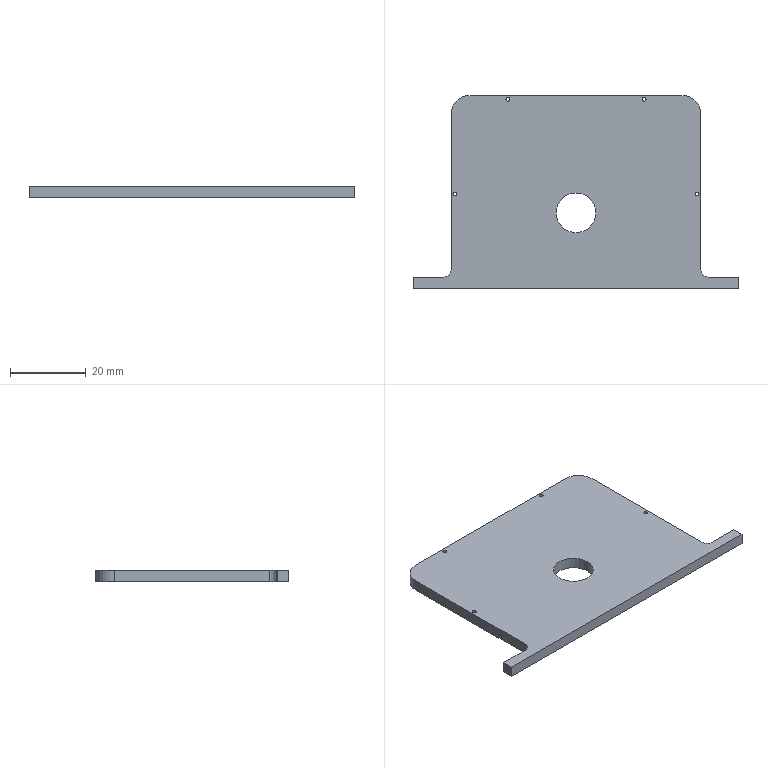Part | SolidWorks | features Extrusion 1 | 1 solid | 24 faces | box 86 x 51 x 3 mm | volume 9982 mm3 | cylinder 14 | plane 10 | commonest cylinder face diameters 1 x8 4 x2 10 x2 10.5 x2
STEP:
#1=CARTESIAN_POINT('',(10.5,25.,3.));
#2=VERTEX_POINT('',#1);
#3=CARTESIAN_POINT('',(11.5,25.,3.));
#4=VERTEX_POINT('',#3);
#5=CARTESIAN_POINT('',(11.,25.,3.));
#6=DIRECTION('',(0.,0.,1.));
#7=DIRECTION('',(1.,0.,0.));
#8=AXIS2_PLACEMENT_3D('',#5,#6,#7);
#9=CIRCLE('',#8,0.5);
#10=EDGE_CURVE('',#2,#4,#9,.T.);
#11=ORIENTED_EDGE('',*,*,#10,.T.);
#12=CARTESIAN_POINT('',(11.5,25.,0.));
#13=VERTEX_POINT('',#12);
#14=CARTESIAN_POINT('',(11.5,25.,3.));
#15=DIRECTION('',(0.,0.,-1.));
#16=VECTOR('',#15,1000.);
#17=LINE('',#14,#16);
#18=EDGE_CURVE('',#4,#13,#17,.T.);
#19=ORIENTED_EDGE('',*,*,#18,.T.);
#20=CARTESIAN_POINT('',(10.5,25.,0.));
#21=VERTEX_POINT('',#20);
#22=CARTESIAN_POINT('',(11.,25.,0.));
#23=DIRECTION('',(0.,0.,1.));
#24=DIRECTION('',(1.,0.,0.));
#25=AXIS2_PLACEMENT_3D('',#22,#23,#24);
#26=CIRCLE('',#25,0.5);
#27=EDGE_CURVE('',#21,#13,#26,.T.);
#28=ORIENTED_EDGE('',*,*,#27,.F.);
#29=CARTESIAN_POINT('',(10.5,25.,3.));
#30=DIRECTION('',(0.,0.,-1.));
#31=VECTOR('',#30,1000.);
#32=LINE('',#29,#31);
#33=EDGE_CURVE('',#2,#21,#32,.T.);
#34=ORIENTED_EDGE('',*,*,#33,.F.);
#35=EDGE_LOOP('',(#11,#19,#28,#34));
#36=FACE_OUTER_BOUND('',#35,.T.);
#37=CARTESIAN_POINT('',(11.,25.,3.));
#38=DIRECTION('',(0.,0.,-1.));
#39=DIRECTION('',(-1.,0.,0.));
#40=AXIS2_PLACEMENT_3D('',#37,#38,#39);
#41=CYLINDRICAL_SURFACE('',#40,0.5);
#42=ADVANCED_FACE('',(#36),#41,.F.);
#43=CARTESIAN_POINT('',(74.5,25.,3.));
#44=VERTEX_POINT('',#43);
#45=CARTESIAN_POINT('',(75.5,25.,3.));
#46=VERTEX_POINT('',#45);
#47=CARTESIAN_POINT('',(75.,25.,3.));
#48=DIRECTION('',(0.,0.,1.));
#49=DIRECTION('',(1.,0.,0.));
#50=AXIS2_PLACEMENT_3D('',#47,#48,#49);
#51=CIRCLE('',#50,0.5);
#52=EDGE_CURVE('',#44,#46,#51,.T.);
#53=ORIENTED_EDGE('',*,*,#52,.T.);
#54=CARTESIAN_POINT('',(75.5,25.,0.));
#55=VERTEX_POINT('',#54);
#56=CARTESIAN_POINT('',(75.5,25.,3.));
#57=DIRECTION('',(0.,0.,-1.));
#58=VECTOR('',#57,1000.);
#59=LINE('',#56,#58);
#60=EDGE_CURVE('',#46,#55,#59,.T.);
#61=ORIENTED_EDGE('',*,*,#60,.T.);
#62=CARTESIAN_POINT('',(74.5,25.,0.));
#63=VERTEX_POINT('',#62);
#64=CARTESIAN_POINT('',(75.,25.,0.));
#65=DIRECTION('',(0.,0.,1.));
#66=DIRECTION('',(1.,0.,0.));
#67=AXIS2_PLACEMENT_3D('',#64,#65,#66);
#68=CIRCLE('',#67,0.5);
#69=EDGE_CURVE('',#63,#55,#68,.T.);
#70=ORIENTED_EDGE('',*,*,#69,.F.);
#71=CARTESIAN_POINT('',(74.5,25.,3.));
#72=DIRECTION('',(0.,0.,-1.));
#73=VECTOR('',#72,1000.);
#74=LINE('',#71,#73);
#75=EDGE_CURVE('',#44,#63,#74,.T.);
#76=ORIENTED_EDGE('',*,*,#75,.F.);
#77=EDGE_LOOP('',(#53,#61,#70,#76));
#78=FACE_OUTER_BOUND('',#77,.T.);
#79=CARTESIAN_POINT('',(75.,25.,3.));
#80=DIRECTION('',(0.,0.,-1.));
#81=DIRECTION('',(-1.,0.,0.));
#82=AXIS2_PLACEMENT_3D('',#79,#80,#81);
#83=CYLINDRICAL_SURFACE('',#82,0.5);
#84=ADVANCED_FACE('',(#78),#83,.F.);
#85=CARTESIAN_POINT('',(60.5,50.,3.));
#86=VERTEX_POINT('',#85);
#87=CARTESIAN_POINT('',(61.5,50.,3.));
#88=VERTEX_POINT('',#87);
#89=CARTESIAN_POINT('',(61.,50.,3.));
#90=DIRECTION('',(0.,0.,1.));
#91=DIRECTION('',(1.,0.,0.));
#92=AXIS2_PLACEMENT_3D('',#89,#90,#91);
#93=CIRCLE('',#92,0.5);
#94=EDGE_CURVE('',#86,#88,#93,.T.);
#95=ORIENTED_EDGE('',*,*,#94,.T.);
#96=CARTESIAN_POINT('',(61.5,50.,0.));
#97=VERTEX_POINT('',#96);
#98=CARTESIAN_POINT('',(61.5,50.,3.));
#99=DIRECTION('',(0.,0.,-1.));
#100=VECTOR('',#99,1000.);
#101=LINE('',#98,#100);
#102=EDGE_CURVE('',#88,#97,#101,.T.);
#103=ORIENTED_EDGE('',*,*,#102,.T.);
#104=CARTESIAN_POINT('',(60.5,50.,0.));
#105=VERTEX_POINT('',#104);
#106=CARTESIAN_POINT('',(61.,50.,0.));
#107=DIRECTION('',(0.,0.,1.));
#108=DIRECTION('',(1.,0.,0.));
#109=AXIS2_PLACEMENT_3D('',#106,#107,#108);
#110=CIRCLE('',#109,0.5);
#111=EDGE_CURVE('',#105,#97,#110,.T.);
#112=ORIENTED_EDGE('',*,*,#111,.F.);
#113=CARTESIAN_POINT('',(60.5,50.,3.));
#114=DIRECTION('',(0.,0.,-1.));
#115=VECTOR('',#114,1000.);
#116=LINE('',#113,#115);
#117=EDGE_CURVE('',#86,#105,#116,.T.);
#118=ORIENTED_EDGE('',*,*,#117,.F.);
#119=EDGE_LOOP('',(#95,#103,#112,#118));
#120=FACE_OUTER_BOUND('',#119,.T.);
#121=CARTESIAN_POINT('',(61.,50.,3.));
#122=DIRECTION('',(0.,0.,-1.));
#123=DIRECTION('',(-1.,0.,0.));
#124=AXIS2_PLACEMENT_3D('',#121,#122,#123);
#125=CYLINDRICAL_SURFACE('',#124,0.5);
#126=ADVANCED_FACE('',(#120),#125,.F.);
#127=CARTESIAN_POINT('',(24.5,50.,3.));
#128=VERTEX_POINT('',#127);
#129=CARTESIAN_POINT('',(25.5,50.,3.));
#130=VERTEX_POINT('',#129);
#131=CARTESIAN_POINT('',(25.,50.,3.));
#132=DIRECTION('',(0.,0.,1.));
#133=DIRECTION('',(1.,0.,0.));
#134=AXIS2_PLACEMENT_3D('',#131,#132,#133);
#135=CIRCLE('',#134,0.5);
#136=EDGE_CURVE('',#128,#130,#135,.T.);
#137=ORIENTED_EDGE('',*,*,#136,.T.);
#138=CARTESIAN_POINT('',(25.5,50.,0.));
#139=VERTEX_POINT('',#138);
#140=CARTESIAN_POINT('',(25.5,50.,3.));
#141=DIRECTION('',(0.,0.,-1.));
#142=VECTOR('',#141,1000.);
#143=LINE('',#140,#142);
#144=EDGE_CURVE('',#130,#139,#143,.T.);
#145=ORIENTED_EDGE('',*,*,#144,.T.);
#146=CARTESIAN_POINT('',(24.5,50.,0.));
#147=VERTEX_POINT('',#146);
#148=CARTESIAN_POINT('',(25.,50.,0.));
#149=DIRECTION('',(0.,0.,1.));
#150=DIRECTION('',(1.,0.,0.));
#151=AXIS2_PLACEMENT_3D('',#148,#149,#150);
#152=CIRCLE('',#151,0.5);
#153=EDGE_CURVE('',#147,#139,#152,.T.);
#154=ORIENTED_EDGE('',*,*,#153,.F.);
#155=CARTESIAN_POINT('',(24.5,50.,3.));
#156=DIRECTION('',(0.,0.,-1.));
#157=VECTOR('',#156,1000.);
#158=LINE('',#155,#157);
#159=EDGE_CURVE('',#128,#147,#158,.T.);
#160=ORIENTED_EDGE('',*,*,#159,.F.);
#161=EDGE_LOOP('',(#137,#145,#154,#160));
#162=FACE_OUTER_BOUND('',#161,.T.);
#163=CARTESIAN_POINT('',(25.,50.,3.));
#164=DIRECTION('',(0.,0.,-1.));
#165=DIRECTION('',(-1.,0.,0.));
#166=AXIS2_PLACEMENT_3D('',#163,#164,#165);
#167=CYLINDRICAL_SURFACE('',#166,0.5);
#168=ADVANCED_FACE('',(#162),#167,.F.);
#169=CARTESIAN_POINT('',(37.75,20.,3.));
#170=VERTEX_POINT('',#169);
#171=CARTESIAN_POINT('',(48.25,20.,3.));
#172=VERTEX_POINT('',#171);
#173=CARTESIAN_POINT('',(43.,20.,3.));
#174=DIRECTION('',(0.,0.,1.));
#175=DIRECTION('',(1.,0.,0.));
#176=AXIS2_PLACEMENT_3D('',#173,#174,#175);
#177=CIRCLE('',#176,5.25);
#178=EDGE_CURVE('',#170,#172,#177,.T.);
#179=ORIENTED_EDGE('',*,*,#178,.T.);
#180=CARTESIAN_POINT('',(48.25,20.,0.));
#181=VERTEX_POINT('',#180);
#182=CARTESIAN_POINT('',(48.25,20.,3.));
#183=DIRECTION('',(0.,0.,-1.));
#184=VECTOR('',#183,1000.);
#185=LINE('',#182,#184);
#186=EDGE_CURVE('',#172,#181,#185,.T.);
#187=ORIENTED_EDGE('',*,*,#186,.T.);
#188=CARTESIAN_POINT('',(37.75,20.,0.));
#189=VERTEX_POINT('',#188);
#190=CARTESIAN_POINT('',(43.,20.,0.));
#191=DIRECTION('',(0.,0.,1.));
#192=DIRECTION('',(1.,0.,0.));
#193=AXIS2_PLACEMENT_3D('',#190,#191,#192);
#194=CIRCLE('',#193,5.25);
#195=EDGE_CURVE('',#189,#181,#194,.T.);
#196=ORIENTED_EDGE('',*,*,#195,.F.);
#197=CARTESIAN_POINT('',(37.75,20.,3.));
#198=DIRECTION('',(0.,0.,-1.));
#199=VECTOR('',#198,1000.);
#200=LINE('',#197,#199);
#201=EDGE_CURVE('',#170,#189,#200,.T.);
#202=ORIENTED_EDGE('',*,*,#201,.F.);
#203=EDGE_LOOP('',(#179,#187,#196,#202));
#204=FACE_OUTER_BOUND('',#203,.T.);
#205=CARTESIAN_POINT('',(43.,20.,3.));
#206=DIRECTION('',(0.,0.,-1.));
#207=DIRECTION('',(-1.,0.,0.));
#208=AXIS2_PLACEMENT_3D('',#205,#206,#207);
#209=CYLINDRICAL_SURFACE('',#208,5.25);
#210=ADVANCED_FACE('',(#204),#209,.F.);
#211=CARTESIAN_POINT('',(0.,0.,3.));
#212=VERTEX_POINT('',#211);
#213=CARTESIAN_POINT('',(86.,0.,3.));
#214=VERTEX_POINT('',#213);
#215=CARTESIAN_POINT('',(86.,0.,3.));
#216=DIRECTION('',(1.,0.,0.));
#217=VECTOR('',#216,1000.);
#218=LINE('',#215,#217);
#219=EDGE_CURVE('',#212,#214,#218,.T.);
#220=ORIENTED_EDGE('',*,*,#219,.T.);
#221=CARTESIAN_POINT('',(86.,3.,3.));
#222=VERTEX_POINT('',#221);
#223=CARTESIAN_POINT('',(86.,0.,3.));
#224=DIRECTION('',(0.,1.,0.));
#225=VECTOR('',#224,1000.);
#226=LINE('',#223,#225);
#227=EDGE_CURVE('',#214,#222,#226,.T.);
#228=ORIENTED_EDGE('',*,*,#227,.T.);
#229=CARTESIAN_POINT('',(78.,3.,3.));
#230=VERTEX_POINT('',#229);
#231=CARTESIAN_POINT('',(86.,3.,3.));
#232=DIRECTION('',(-1.,0.,0.));
#233=VECTOR('',#232,1000.);
#234=LINE('',#231,#233);
#235=EDGE_CURVE('',#222,#230,#234,.T.);
#236=ORIENTED_EDGE('',*,*,#235,.T.);
#237=CARTESIAN_POINT('',(76.,5.,3.));
#238=VERTEX_POINT('',#237);
#239=CARTESIAN_POINT('',(78.,5.,3.));
#240=DIRECTION('',(0.,0.,-1.));
#241=DIRECTION('',(-1.,0.,0.));
#242=AXIS2_PLACEMENT_3D('',#239,#240,#241);
#243=CIRCLE('',#242,2.);
#244=EDGE_CURVE('',#230,#238,#243,.T.);
#245=ORIENTED_EDGE('',*,*,#244,.T.);
#246=CARTESIAN_POINT('',(76.,46.,3.));
#247=VERTEX_POINT('',#246);
#248=CARTESIAN_POINT('',(76.,5.,3.));
#249=DIRECTION('',(0.,1.,0.));
#250=VECTOR('',#249,1000.);
#251=LINE('',#248,#250);
#252=EDGE_CURVE('',#238,#247,#251,.T.);
#253=ORIENTED_EDGE('',*,*,#252,.T.);
#254=CARTESIAN_POINT('',(71.,51.,3.));
#255=VERTEX_POINT('',#254);
#256=CARTESIAN_POINT('',(71.,46.,3.));
#257=DIRECTION('',(0.,0.,1.));
#258=DIRECTION('',(1.,0.,0.));
#259=AXIS2_PLACEMENT_3D('',#256,#257,#258);
#260=CIRCLE('',#259,5.);
#261=EDGE_CURVE('',#247,#255,#260,.T.);
#262=ORIENTED_EDGE('',*,*,#261,.T.);
#263=CARTESIAN_POINT('',(15.,51.,3.));
#264=VERTEX_POINT('',#263);
#265=CARTESIAN_POINT('',(71.,51.,3.));
#266=DIRECTION('',(-1.,0.,0.));
#267=VECTOR('',#266,1000.);
#268=LINE('',#265,#267);
#269=EDGE_CURVE('',#255,#264,#268,.T.);
#270=ORIENTED_EDGE('',*,*,#269,.T.);
#271=CARTESIAN_POINT('',(10.,46.,3.));
#272=VERTEX_POINT('',#271);
#273=CARTESIAN_POINT('',(15.,46.,3.));
#274=DIRECTION('',(0.,0.,1.));
#275=DIRECTION('',(1.,0.,0.));
#276=AXIS2_PLACEMENT_3D('',#273,#274,#275);
#277=CIRCLE('',#276,5.);
#278=EDGE_CURVE('',#264,#272,#277,.T.);
#279=ORIENTED_EDGE('',*,*,#278,.T.);
#280=CARTESIAN_POINT('',(10.,5.,3.));
#281=VERTEX_POINT('',#280);
#282=CARTESIAN_POINT('',(10.,46.,3.));
#283=DIRECTION('',(0.,-1.,0.));
#284=VECTOR('',#283,1000.);
#285=LINE('',#282,#284);
#286=EDGE_CURVE('',#272,#281,#285,.T.);
#287=ORIENTED_EDGE('',*,*,#286,.T.);
#288=CARTESIAN_POINT('',(8.,3.,3.));
#289=VERTEX_POINT('',#288);
#290=CARTESIAN_POINT('',(8.,5.,3.));
#291=DIRECTION('',(0.,0.,-1.));
#292=DIRECTION('',(-1.,0.,0.));
#293=AXIS2_PLACEMENT_3D('',#290,#291,#292);
#294=CIRCLE('',#293,2.);
#295=EDGE_CURVE('',#281,#289,#294,.T.);
#296=ORIENTED_EDGE('',*,*,#295,.T.);
#297=CARTESIAN_POINT('',(0.,3.,3.));
#298=VERTEX_POINT('',#297);
#299=CARTESIAN_POINT('',(8.,3.,3.));
#300=DIRECTION('',(-1.,0.,0.));
#301=VECTOR('',#300,1000.);
#302=LINE('',#299,#301);
#303=EDGE_CURVE('',#289,#298,#302,.T.);
#304=ORIENTED_EDGE('',*,*,#303,.T.);
#305=CARTESIAN_POINT('',(0.,3.,3.));
#306=DIRECTION('',(0.,-1.,0.));
#307=VECTOR('',#306,1000.);
#308=LINE('',#305,#307);
#309=EDGE_CURVE('',#298,#212,#308,.T.);
#310=ORIENTED_EDGE('',*,*,#309,.T.);
#311=EDGE_LOOP('',(#220,#228,#236,#245,#253,#262,#270,#279,#287,#296,#304,#310));
#312=FACE_OUTER_BOUND('',#311,.T.);
#313=ORIENTED_EDGE('',*,*,#178,.F.);
#314=CARTESIAN_POINT('',(43.,20.,3.));
#315=DIRECTION('',(0.,0.,1.));
#316=DIRECTION('',(1.,0.,0.));
#317=AXIS2_PLACEMENT_3D('',#314,#315,#316);
#318=CIRCLE('',#317,5.25);
#319=EDGE_CURVE('',#172,#170,#318,.T.);
#320=ORIENTED_EDGE('',*,*,#319,.F.);
#321=EDGE_LOOP('',(#313,#320));
#322=FACE_BOUND('',#321,.T.);
#323=ORIENTED_EDGE('',*,*,#136,.F.);
#324=CARTESIAN_POINT('',(25.,50.,3.));
#325=DIRECTION('',(0.,0.,1.));
#326=DIRECTION('',(1.,0.,0.));
#327=AXIS2_PLACEMENT_3D('',#324,#325,#326);
#328=CIRCLE('',#327,0.5);
#329=EDGE_CURVE('',#130,#128,#328,.T.);
#330=ORIENTED_EDGE('',*,*,#329,.F.);
#331=EDGE_LOOP('',(#323,#330));
#332=FACE_BOUND('',#331,.T.);
#333=ORIENTED_EDGE('',*,*,#94,.F.);
#334=CARTESIAN_POINT('',(61.,50.,3.));
#335=DIRECTION('',(0.,0.,1.));
#336=DIRECTION('',(1.,0.,0.));
#337=AXIS2_PLACEMENT_3D('',#334,#335,#336);
#338=CIRCLE('',#337,0.5);
#339=EDGE_CURVE('',#88,#86,#338,.T.);
#340=ORIENTED_EDGE('',*,*,#339,.F.);
#341=EDGE_LOOP('',(#333,#340));
#342=FACE_BOUND('',#341,.T.);
#343=ORIENTED_EDGE('',*,*,#52,.F.);
#344=CARTESIAN_POINT('',(75.,25.,3.));
#345=DIRECTION('',(0.,0.,1.));
#346=DIRECTION('',(1.,0.,0.));
#347=AXIS2_PLACEMENT_3D('',#344,#345,#346);
#348=CIRCLE('',#347,0.5);
#349=EDGE_CURVE('',#46,#44,#348,.T.);
#350=ORIENTED_EDGE('',*,*,#349,.F.);
#351=EDGE_LOOP('',(#343,#350));
#352=FACE_BOUND('',#351,.T.);
#353=ORIENTED_EDGE('',*,*,#10,.F.);
#354=CARTESIAN_POINT('',(11.,25.,3.));
#355=DIRECTION('',(0.,0.,1.));
#356=DIRECTION('',(1.,0.,0.));
#357=AXIS2_PLACEMENT_3D('',#354,#355,#356);
#358=CIRCLE('',#357,0.5);
#359=EDGE_CURVE('',#4,#2,#358,.T.);
#360=ORIENTED_EDGE('',*,*,#359,.F.);
#361=EDGE_LOOP('',(#353,#360));
#362=FACE_BOUND('',#361,.T.);
#363=CARTESIAN_POINT('',(8.,5.,3.));
#364=DIRECTION('',(0.,0.,-1.));
#365=DIRECTION('',(-1.,0.,0.));
#366=AXIS2_PLACEMENT_3D('',#363,#364,#365);
#367=PLANE('',#366);
#368=ADVANCED_FACE('',(#312,#322,#332,#342,#352,#362),#367,.F.);
#369=ORIENTED_EDGE('',*,*,#69,.T.);
#370=CARTESIAN_POINT('',(75.,25.,0.));
#371=DIRECTION('',(0.,0.,1.));
#372=DIRECTION('',(1.,0.,0.));
#373=AXIS2_PLACEMENT_3D('',#370,#371,#372);
#374=CIRCLE('',#373,0.5);
#375=EDGE_CURVE('',#55,#63,#374,.T.);
#376=ORIENTED_EDGE('',*,*,#375,.T.);
#377=EDGE_LOOP('',(#369,#376));
#378=FACE_BOUND('',#377,.T.);
#379=ORIENTED_EDGE('',*,*,#153,.T.);
#380=CARTESIAN_POINT('',(25.,50.,0.));
#381=DIRECTION('',(0.,0.,1.));
#382=DIRECTION('',(1.,0.,0.));
#383=AXIS2_PLACEMENT_3D('',#380,#381,#382);
#384=CIRCLE('',#383,0.5);
#385=EDGE_CURVE('',#139,#147,#384,.T.);
#386=ORIENTED_EDGE('',*,*,#385,.T.);
#387=EDGE_LOOP('',(#379,#386));
#388=FACE_BOUND('',#387,.T.);
#389=CARTESIAN_POINT('',(0.,0.,0.));
#390=VERTEX_POINT('',#389);
#391=CARTESIAN_POINT('',(86.,0.,0.));
#392=VERTEX_POINT('',#391);
#393=CARTESIAN_POINT('',(86.,0.,0.));
#394=DIRECTION('',(1.,0.,0.));
#395=VECTOR('',#394,1000.);
#396=LINE('',#393,#395);
#397=EDGE_CURVE('',#390,#392,#396,.T.);
#398=ORIENTED_EDGE('',*,*,#397,.F.);
#399=CARTESIAN_POINT('',(0.,3.,0.));
#400=VERTEX_POINT('',#399);
#401=CARTESIAN_POINT('',(0.,3.,0.));
#402=DIRECTION('',(0.,-1.,0.));
#403=VECTOR('',#402,1000.);
#404=LINE('',#401,#403);
#405=EDGE_CURVE('',#400,#390,#404,.T.);
#406=ORIENTED_EDGE('',*,*,#405,.F.);
#407=CARTESIAN_POINT('',(8.,3.,0.));
#408=VERTEX_POINT('',#407);
#409=CARTESIAN_POINT('',(8.,3.,0.));
#410=DIRECTION('',(-1.,0.,0.));
#411=VECTOR('',#410,1000.);
#412=LINE('',#409,#411);
#413=EDGE_CURVE('',#408,#400,#412,.T.);
#414=ORIENTED_EDGE('',*,*,#413,.F.);
#415=CARTESIAN_POINT('',(10.,5.,0.));
#416=VERTEX_POINT('',#415);
#417=CARTESIAN_POINT('',(8.,5.,0.));
#418=DIRECTION('',(0.,0.,-1.));
#419=DIRECTION('',(-1.,0.,0.));
#420=AXIS2_PLACEMENT_3D('',#417,#418,#419);
#421=CIRCLE('',#420,2.);
#422=EDGE_CURVE('',#416,#408,#421,.T.);
#423=ORIENTED_EDGE('',*,*,#422,.F.);
#424=CARTESIAN_POINT('',(10.,46.,0.));
#425=VERTEX_POINT('',#424);
#426=CARTESIAN_POINT('',(10.,46.,0.));
#427=DIRECTION('',(0.,-1.,0.));
#428=VECTOR('',#427,1000.);
#429=LINE('',#426,#428);
#430=EDGE_CURVE('',#425,#416,#429,.T.);
#431=ORIENTED_EDGE('',*,*,#430,.F.);
#432=CARTESIAN_POINT('',(15.,51.,0.));
#433=VERTEX_POINT('',#432);
#434=CARTESIAN_POINT('',(15.,46.,0.));
#435=DIRECTION('',(0.,0.,1.));
#436=DIRECTION('',(1.,0.,0.));
#437=AXIS2_PLACEMENT_3D('',#434,#435,#436);
#438=CIRCLE('',#437,5.);
#439=EDGE_CURVE('',#433,#425,#438,.T.);
#440=ORIENTED_EDGE('',*,*,#439,.F.);
#441=CARTESIAN_POINT('',(71.,51.,0.));
#442=VERTEX_POINT('',#441);
#443=CARTESIAN_POINT('',(71.,51.,0.));
#444=DIRECTION('',(-1.,0.,0.));
#445=VECTOR('',#444,1000.);
#446=LINE('',#443,#445);
#447=EDGE_CURVE('',#442,#433,#446,.T.);
#448=ORIENTED_EDGE('',*,*,#447,.F.);
#449=CARTESIAN_POINT('',(76.,46.,0.));
#450=VERTEX_POINT('',#449);
#451=CARTESIAN_POINT('',(71.,46.,0.));
#452=DIRECTION('',(0.,0.,1.));
#453=DIRECTION('',(1.,0.,0.));
#454=AXIS2_PLACEMENT_3D('',#451,#452,#453);
#455=CIRCLE('',#454,5.);
#456=EDGE_CURVE('',#450,#442,#455,.T.);
#457=ORIENTED_EDGE('',*,*,#456,.F.);
#458=CARTESIAN_POINT('',(76.,5.,0.));
#459=VERTEX_POINT('',#458);
#460=CARTESIAN_POINT('',(76.,5.,0.));
#461=DIRECTION('',(0.,1.,0.));
#462=VECTOR('',#461,1000.);
#463=LINE('',#460,#462);
#464=EDGE_CURVE('',#459,#450,#463,.T.);
#465=ORIENTED_EDGE('',*,*,#464,.F.);
#466=CARTESIAN_POINT('',(78.,3.,0.));
#467=VERTEX_POINT('',#466);
#468=CARTESIAN_POINT('',(78.,5.,0.));
#469=DIRECTION('',(0.,0.,-1.));
#470=DIRECTION('',(-1.,0.,0.));
#471=AXIS2_PLACEMENT_3D('',#468,#469,#470);
#472=CIRCLE('',#471,2.);
#473=EDGE_CURVE('',#467,#459,#472,.T.);
#474=ORIENTED_EDGE('',*,*,#473,.F.);
#475=CARTESIAN_POINT('',(86.,3.,0.));
#476=VERTEX_POINT('',#475);
#477=CARTESIAN_POINT('',(86.,3.,0.));
#478=DIRECTION('',(-1.,0.,0.));
#479=VECTOR('',#478,1000.);
#480=LINE('',#477,#479);
#481=EDGE_CURVE('',#476,#467,#480,.T.);
#482=ORIENTED_EDGE('',*,*,#481,.F.);
#483=CARTESIAN_POINT('',(86.,0.,0.));
#484=DIRECTION('',(0.,1.,0.));
#485=VECTOR('',#484,1000.);
#486=LINE('',#483,#485);
#487=EDGE_CURVE('',#392,#476,#486,.T.);
#488=ORIENTED_EDGE('',*,*,#487,.F.);
#489=EDGE_LOOP('',(#398,#406,#414,#423,#431,#440,#448,#457,#465,#474,#482,#488));
#490=FACE_OUTER_BOUND('',#489,.T.);
#491=ORIENTED_EDGE('',*,*,#195,.T.);
#492=CARTESIAN_POINT('',(43.,20.,0.));
#493=DIRECTION('',(0.,0.,1.));
#494=DIRECTION('',(1.,0.,0.));
#495=AXIS2_PLACEMENT_3D('',#492,#493,#494);
#496=CIRCLE('',#495,5.25);
#497=EDGE_CURVE('',#181,#189,#496,.T.);
#498=ORIENTED_EDGE('',*,*,#497,.T.);
#499=EDGE_LOOP('',(#491,#498));
#500=FACE_BOUND('',#499,.T.);
#501=ORIENTED_EDGE('',*,*,#111,.T.);
#502=CARTESIAN_POINT('',(61.,50.,0.));
#503=DIRECTION('',(0.,0.,1.));
#504=DIRECTION('',(1.,0.,0.));
#505=AXIS2_PLACEMENT_3D('',#502,#503,#504);
#506=CIRCLE('',#505,0.5);
#507=EDGE_CURVE('',#97,#105,#506,.T.);
#508=ORIENTED_EDGE('',*,*,#507,.T.);
#509=EDGE_LOOP('',(#501,#508));
#510=FACE_BOUND('',#509,.T.);
#511=ORIENTED_EDGE('',*,*,#27,.T.);
#512=CARTESIAN_POINT('',(11.,25.,0.));
#513=DIRECTION('',(0.,0.,1.));
#514=DIRECTION('',(1.,0.,0.));
#515=AXIS2_PLACEMENT_3D('',#512,#513,#514);
#516=CIRCLE('',#515,0.5);
#517=EDGE_CURVE('',#13,#21,#516,.T.);
#518=ORIENTED_EDGE('',*,*,#517,.T.);
#519=EDGE_LOOP('',(#511,#518));
#520=FACE_BOUND('',#519,.T.);
#521=CARTESIAN_POINT('',(8.,5.,0.));
#522=DIRECTION('',(0.,0.,-1.));
#523=DIRECTION('',(-1.,0.,0.));
#524=AXIS2_PLACEMENT_3D('',#521,#522,#523);
#525=PLANE('',#524);
#526=ADVANCED_FACE('',(#378,#388,#490,#500,#510,#520),#525,.T.);
#527=ORIENTED_EDGE('',*,*,#397,.T.);
#528=CARTESIAN_POINT('',(86.,0.,3.));
#529=DIRECTION('',(0.,0.,-1.));
#530=VECTOR('',#529,1000.);
#531=LINE('',#528,#530);
#532=EDGE_CURVE('',#214,#392,#531,.T.);
#533=ORIENTED_EDGE('',*,*,#532,.F.);
#534=ORIENTED_EDGE('',*,*,#219,.F.);
#535=CARTESIAN_POINT('',(0.,0.,3.));
#536=DIRECTION('',(0.,0.,-1.));
#537=VECTOR('',#536,1000.);
#538=LINE('',#535,#537);
#539=EDGE_CURVE('',#212,#390,#538,.T.);
#540=ORIENTED_EDGE('',*,*,#539,.T.);
#541=EDGE_LOOP('',(#527,#533,#534,#540));
#542=FACE_OUTER_BOUND('',#541,.T.);
#543=CARTESIAN_POINT('',(86.,0.,3.));
#544=DIRECTION('',(0.,1.,0.));
#545=DIRECTION('',(0.,0.,1.));
#546=AXIS2_PLACEMENT_3D('',#543,#544,#545);
#547=PLANE('',#546);
#548=ADVANCED_FACE('',(#542),#547,.F.);
#549=ORIENTED_EDGE('',*,*,#487,.T.);
#550=CARTESIAN_POINT('',(86.,3.,3.));
#551=DIRECTION('',(0.,0.,-1.));
#552=VECTOR('',#551,1000.);
#553=LINE('',#550,#552);
#554=EDGE_CURVE('',#222,#476,#553,.T.);
#555=ORIENTED_EDGE('',*,*,#554,.F.);
#556=ORIENTED_EDGE('',*,*,#227,.F.);
#557=ORIENTED_EDGE('',*,*,#532,.T.);
#558=EDGE_LOOP('',(#549,#555,#556,#557));
#559=FACE_OUTER_BOUND('',#558,.T.);
#560=CARTESIAN_POINT('',(86.,0.,3.));
#561=DIRECTION('',(-1.,0.,0.));
#562=DIRECTION('',(0.,-1.,0.));
#563=AXIS2_PLACEMENT_3D('',#560,#561,#562);
#564=PLANE('',#563);
#565=ADVANCED_FACE('',(#559),#564,.F.);
#566=ORIENTED_EDGE('',*,*,#481,.T.);
#567=CARTESIAN_POINT('',(78.,3.,3.));
#568=DIRECTION('',(0.,0.,-1.));
#569=VECTOR('',#568,1000.);
#570=LINE('',#567,#569);
#571=EDGE_CURVE('',#230,#467,#570,.T.);
#572=ORIENTED_EDGE('',*,*,#571,.F.);
#573=ORIENTED_EDGE('',*,*,#235,.F.);
#574=ORIENTED_EDGE('',*,*,#554,.T.);
#575=EDGE_LOOP('',(#566,#572,#573,#574));
#576=FACE_OUTER_BOUND('',#575,.T.);
#577=CARTESIAN_POINT('',(86.,3.,3.));
#578=DIRECTION('',(0.,-1.,0.));
#579=DIRECTION('',(1.,0.,0.));
#580=AXIS2_PLACEMENT_3D('',#577,#578,#579);
#581=PLANE('',#580);
#582=ADVANCED_FACE('',(#576),#581,.F.);
#583=ORIENTED_EDGE('',*,*,#473,.T.);
#584=CARTESIAN_POINT('',(76.,5.,3.));
#585=DIRECTION('',(0.,0.,-1.));
#586=VECTOR('',#585,1000.);
#587=LINE('',#584,#586);
#588=EDGE_CURVE('',#238,#459,#587,.T.);
#589=ORIENTED_EDGE('',*,*,#588,.F.);
#590=ORIENTED_EDGE('',*,*,#244,.F.);
#591=ORIENTED_EDGE('',*,*,#571,.T.);
#592=EDGE_LOOP('',(#583,#589,#590,#591));
#593=FACE_OUTER_BOUND('',#592,.T.);
#594=CARTESIAN_POINT('',(78.,5.,3.));
#595=DIRECTION('',(0.,0.,-1.));
#596=DIRECTION('',(-1.,0.,0.));
#597=AXIS2_PLACEMENT_3D('',#594,#595,#596);
#598=CYLINDRICAL_SURFACE('',#597,2.);
#599=ADVANCED_FACE('',(#593),#598,.F.);
#600=ORIENTED_EDGE('',*,*,#464,.T.);
#601=CARTESIAN_POINT('',(76.,46.,3.));
#602=DIRECTION('',(0.,0.,-1.));
#603=VECTOR('',#602,1000.);
#604=LINE('',#601,#603);
#605=EDGE_CURVE('',#247,#450,#604,.T.);
#606=ORIENTED_EDGE('',*,*,#605,.F.);
#607=ORIENTED_EDGE('',*,*,#252,.F.);
#608=ORIENTED_EDGE('',*,*,#588,.T.);
#609=EDGE_LOOP('',(#600,#606,#607,#608));
#610=FACE_OUTER_BOUND('',#609,.T.);
#611=CARTESIAN_POINT('',(76.,5.,3.));
#612=DIRECTION('',(-1.,0.,0.));
#613=DIRECTION('',(0.,-1.,0.));
#614=AXIS2_PLACEMENT_3D('',#611,#612,#613);
#615=PLANE('',#614);
#616=ADVANCED_FACE('',(#610),#615,.F.);
#617=ORIENTED_EDGE('',*,*,#456,.T.);
#618=CARTESIAN_POINT('',(71.,51.,3.));
#619=DIRECTION('',(0.,0.,-1.));
#620=VECTOR('',#619,1000.);
#621=LINE('',#618,#620);
#622=EDGE_CURVE('',#255,#442,#621,.T.);
#623=ORIENTED_EDGE('',*,*,#622,.F.);
#624=ORIENTED_EDGE('',*,*,#261,.F.);
#625=ORIENTED_EDGE('',*,*,#605,.T.);
#626=EDGE_LOOP('',(#617,#623,#624,#625));
#627=FACE_OUTER_BOUND('',#626,.T.);
#628=CARTESIAN_POINT('',(71.,46.,3.));
#629=DIRECTION('',(0.,0.,-1.));
#630=DIRECTION('',(-1.,0.,0.));
#631=AXIS2_PLACEMENT_3D('',#628,#629,#630);
#632=CYLINDRICAL_SURFACE('',#631,5.);
#633=ADVANCED_FACE('',(#627),#632,.T.);
#634=ORIENTED_EDGE('',*,*,#447,.T.);
#635=CARTESIAN_POINT('',(15.,51.,3.));
#636=DIRECTION('',(0.,0.,-1.));
#637=VECTOR('',#636,1000.);
#638=LINE('',#635,#637);
#639=EDGE_CURVE('',#264,#433,#638,.T.);
#640=ORIENTED_EDGE('',*,*,#639,.F.);
#641=ORIENTED_EDGE('',*,*,#269,.F.);
#642=ORIENTED_EDGE('',*,*,#622,.T.);
#643=EDGE_LOOP('',(#634,#640,#641,#642));
#644=FACE_OUTER_BOUND('',#643,.T.);
#645=CARTESIAN_POINT('',(71.,51.,3.));
#646=DIRECTION('',(0.,-1.,0.));
#647=DIRECTION('',(1.,0.,0.));
#648=AXIS2_PLACEMENT_3D('',#645,#646,#647);
#649=PLANE('',#648);
#650=ADVANCED_FACE('',(#644),#649,.F.);
#651=ORIENTED_EDGE('',*,*,#439,.T.);
#652=CARTESIAN_POINT('',(10.,46.,3.));
#653=DIRECTION('',(0.,0.,-1.));
#654=VECTOR('',#653,1000.);
#655=LINE('',#652,#654);
#656=EDGE_CURVE('',#272,#425,#655,.T.);
#657=ORIENTED_EDGE('',*,*,#656,.F.);
#658=ORIENTED_EDGE('',*,*,#278,.F.);
#659=ORIENTED_EDGE('',*,*,#639,.T.);
#660=EDGE_LOOP('',(#651,#657,#658,#659));
#661=FACE_OUTER_BOUND('',#660,.T.);
#662=CARTESIAN_POINT('',(15.,46.,3.));
#663=DIRECTION('',(0.,0.,-1.));
#664=DIRECTION('',(-1.,0.,0.));
#665=AXIS2_PLACEMENT_3D('',#662,#663,#664);
#666=CYLINDRICAL_SURFACE('',#665,5.);
#667=ADVANCED_FACE('',(#661),#666,.T.);
#668=ORIENTED_EDGE('',*,*,#430,.T.);
#669=CARTESIAN_POINT('',(10.,5.,3.));
#670=DIRECTION('',(0.,0.,-1.));
#671=VECTOR('',#670,1000.);
#672=LINE('',#669,#671);
#673=EDGE_CURVE('',#281,#416,#672,.T.);
#674=ORIENTED_EDGE('',*,*,#673,.F.);
#675=ORIENTED_EDGE('',*,*,#286,.F.);
#676=ORIENTED_EDGE('',*,*,#656,.T.);
#677=EDGE_LOOP('',(#668,#674,#675,#676));
#678=FACE_OUTER_BOUND('',#677,.T.);
#679=CARTESIAN_POINT('',(10.,46.,3.));
#680=DIRECTION('',(1.,0.,0.));
#681=DIRECTION('',(0.,1.,0.));
#682=AXIS2_PLACEMENT_3D('',#679,#680,#681);
#683=PLANE('',#682);
#684=ADVANCED_FACE('',(#678),#683,.F.);
#685=ORIENTED_EDGE('',*,*,#422,.T.);
#686=CARTESIAN_POINT('',(8.,3.,3.));
#687=DIRECTION('',(0.,0.,-1.));
#688=VECTOR('',#687,1000.);
#689=LINE('',#686,#688);
#690=EDGE_CURVE('',#289,#408,#689,.T.);
#691=ORIENTED_EDGE('',*,*,#690,.F.);
#692=ORIENTED_EDGE('',*,*,#295,.F.);
#693=ORIENTED_EDGE('',*,*,#673,.T.);
#694=EDGE_LOOP('',(#685,#691,#692,#693));
#695=FACE_OUTER_BOUND('',#694,.T.);
#696=CARTESIAN_POINT('',(8.,5.,3.));
#697=DIRECTION('',(0.,0.,-1.));
#698=DIRECTION('',(-1.,0.,0.));
#699=AXIS2_PLACEMENT_3D('',#696,#697,#698);
#700=CYLINDRICAL_SURFACE('',#699,2.);
#701=ADVANCED_FACE('',(#695),#700,.F.);
#702=ORIENTED_EDGE('',*,*,#413,.T.);
#703=CARTESIAN_POINT('',(0.,3.,3.));
#704=DIRECTION('',(0.,0.,-1.));
#705=VECTOR('',#704,1000.);
#706=LINE('',#703,#705);
#707=EDGE_CURVE('',#298,#400,#706,.T.);
#708=ORIENTED_EDGE('',*,*,#707,.F.);
#709=ORIENTED_EDGE('',*,*,#303,.F.);
#710=ORIENTED_EDGE('',*,*,#690,.T.);
#711=EDGE_LOOP('',(#702,#708,#709,#710));
#712=FACE_OUTER_BOUND('',#711,.T.);
#713=CARTESIAN_POINT('',(8.,3.,3.));
#714=DIRECTION('',(0.,-1.,0.));
#715=DIRECTION('',(0.,0.,-1.));
#716=AXIS2_PLACEMENT_3D('',#713,#714,#715);
#717=PLANE('',#716);
#718=ADVANCED_FACE('',(#712),#717,.F.);
#719=ORIENTED_EDGE('',*,*,#405,.T.);
#720=ORIENTED_EDGE('',*,*,#539,.F.);
#721=ORIENTED_EDGE('',*,*,#309,.F.);
#722=ORIENTED_EDGE('',*,*,#707,.T.);
#723=EDGE_LOOP('',(#719,#720,#721,#722));
#724=FACE_OUTER_BOUND('',#723,.T.);
#725=CARTESIAN_POINT('',(0.,3.,3.));
#726=DIRECTION('',(1.,0.,0.));
#727=DIRECTION('',(0.,1.,0.));
#728=AXIS2_PLACEMENT_3D('',#725,#726,#727);
#729=PLANE('',#728);
#730=ADVANCED_FACE('',(#724),#729,.F.);
#731=ORIENTED_EDGE('',*,*,#186,.F.);
#732=ORIENTED_EDGE('',*,*,#319,.T.);
#733=ORIENTED_EDGE('',*,*,#201,.T.);
#734=ORIENTED_EDGE('',*,*,#497,.F.);
#735=EDGE_LOOP('',(#731,#732,#733,#734));
#736=FACE_OUTER_BOUND('',#735,.T.);
#737=CARTESIAN_POINT('',(43.,20.,3.));
#738=DIRECTION('',(0.,0.,-1.));
#739=DIRECTION('',(-1.,0.,0.));
#740=AXIS2_PLACEMENT_3D('',#737,#738,#739);
#741=CYLINDRICAL_SURFACE('',#740,5.25);
#742=ADVANCED_FACE('',(#736),#741,.F.);
#743=ORIENTED_EDGE('',*,*,#144,.F.);
#744=ORIENTED_EDGE('',*,*,#329,.T.);
#745=ORIENTED_EDGE('',*,*,#159,.T.);
#746=ORIENTED_EDGE('',*,*,#385,.F.);
#747=EDGE_LOOP('',(#743,#744,#745,#746));
#748=FACE_OUTER_BOUND('',#747,.T.);
#749=CARTESIAN_POINT('',(25.,50.,3.));
#750=DIRECTION('',(0.,0.,-1.));
#751=DIRECTION('',(-1.,0.,0.));
#752=AXIS2_PLACEMENT_3D('',#749,#750,#751);
#753=CYLINDRICAL_SURFACE('',#752,0.5);
#754=ADVANCED_FACE('',(#748),#753,.F.);
#755=ORIENTED_EDGE('',*,*,#102,.F.);
#756=ORIENTED_EDGE('',*,*,#339,.T.);
#757=ORIENTED_EDGE('',*,*,#117,.T.);
#758=ORIENTED_EDGE('',*,*,#507,.F.);
#759=EDGE_LOOP('',(#755,#756,#757,#758));
#760=FACE_OUTER_BOUND('',#759,.T.);
#761=CARTESIAN_POINT('',(61.,50.,3.));
#762=DIRECTION('',(0.,0.,-1.));
#763=DIRECTION('',(-1.,0.,0.));
#764=AXIS2_PLACEMENT_3D('',#761,#762,#763);
#765=CYLINDRICAL_SURFACE('',#764,0.5);
#766=ADVANCED_FACE('',(#760),#765,.F.);
#767=ORIENTED_EDGE('',*,*,#60,.F.);
#768=ORIENTED_EDGE('',*,*,#349,.T.);
#769=ORIENTED_EDGE('',*,*,#75,.T.);
#770=ORIENTED_EDGE('',*,*,#375,.F.);
#771=EDGE_LOOP('',(#767,#768,#769,#770));
#772=FACE_OUTER_BOUND('',#771,.T.);
#773=CARTESIAN_POINT('',(75.,25.,3.));
#774=DIRECTION('',(0.,0.,-1.));
#775=DIRECTION('',(-1.,0.,0.));
#776=AXIS2_PLACEMENT_3D('',#773,#774,#775);
#777=CYLINDRICAL_SURFACE('',#776,0.5);
#778=ADVANCED_FACE('',(#772),#777,.F.);
#779=ORIENTED_EDGE('',*,*,#18,.F.);
#780=ORIENTED_EDGE('',*,*,#359,.T.);
#781=ORIENTED_EDGE('',*,*,#33,.T.);
#782=ORIENTED_EDGE('',*,*,#517,.F.);
#783=EDGE_LOOP('',(#779,#780,#781,#782));
#784=FACE_OUTER_BOUND('',#783,.T.);
#785=CARTESIAN_POINT('',(11.,25.,3.));
#786=DIRECTION('',(0.,0.,-1.));
#787=DIRECTION('',(-1.,0.,0.));
#788=AXIS2_PLACEMENT_3D('',#785,#786,#787);
#789=CYLINDRICAL_SURFACE('',#788,0.5);
#790=ADVANCED_FACE('',(#784),#789,.F.);
#791=CLOSED_SHELL('',(#42,#84,#126,#168,#210,#368,#526,#548,#565,#582,#599,#616,#633,#650,#667,#684,#701,#718,#730,#742,#754,#766,#778,#790));
#792=MANIFOLD_SOLID_BREP('',#791);
#793=CARTESIAN_POINT('',(0.,0.,0.));
#794=DIRECTION('',(0.,0.,1.));
#795=DIRECTION('',(1.,0.,0.));
#796=AXIS2_PLACEMENT_3D('',#793,#794,#795);
#797=(LENGTH_UNIT()NAMED_UNIT(*)SI_UNIT(.MILLI.,.METRE.));
#798=UNCERTAINTY_MEASURE_WITH_UNIT(LENGTH_MEASURE(0.00001),#797,'','');
#799=(NAMED_UNIT(*)PLANE_ANGLE_UNIT()SI_UNIT($,.RADIAN.));
#800=(NAMED_UNIT(*)SI_UNIT($,.STERADIAN.)SOLID_ANGLE_UNIT());
#801=(GEOMETRIC_REPRESENTATION_CONTEXT(3)GLOBAL_UNCERTAINTY_ASSIGNED_CONTEXT((#798))GLOBAL_UNIT_ASSIGNED_CONTEXT((#797,#799,#800))REPRESENTATION_CONTEXT('',''));
#802=ADVANCED_BREP_SHAPE_REPRESENTATION('',(#792,#796),#801);